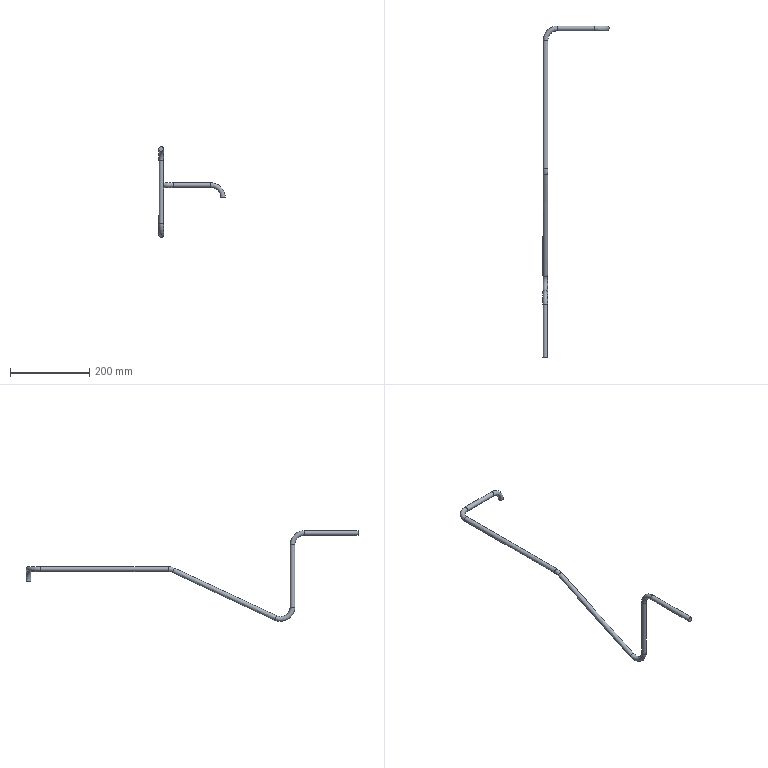Part | NX | features solid 2 | 1 solid | 12 faces | box 167 x 836 x 228.633 mm | volume 136410 mm3 | torus 5 | cylinder 4 | plane 2 | spline 1 | commonest cylinder face diameters 12 x4